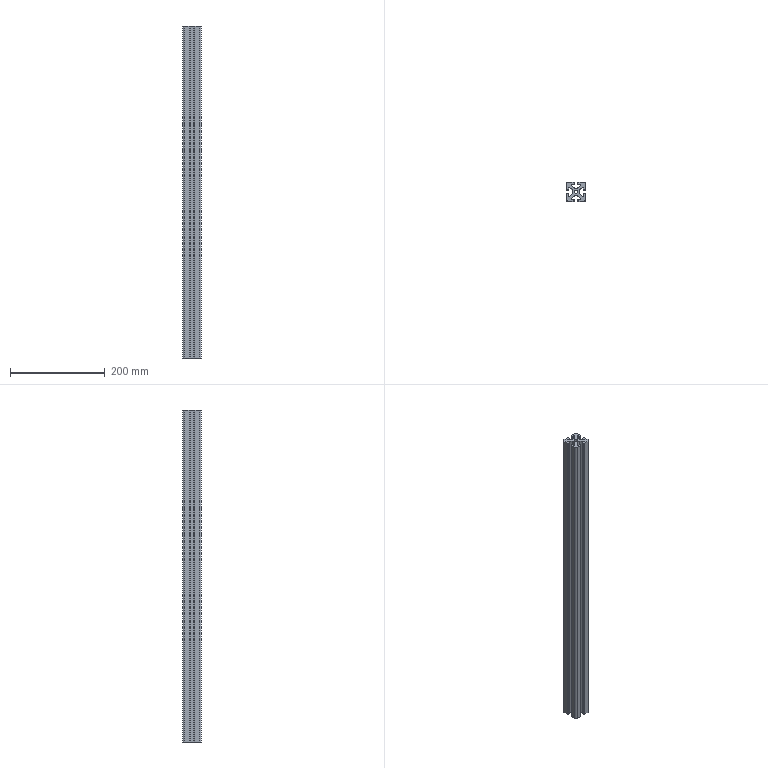Part | SolidWorks | features Extrusion 1 | 1 solid | 78 faces | box 40 x 40 x 700 mm | volume 665465 mm3 | cylinder 48 | plane 30 | commonest cylinder face diameters 2 x26 4 x8 49.184 x8 8 x4 6.8 x2